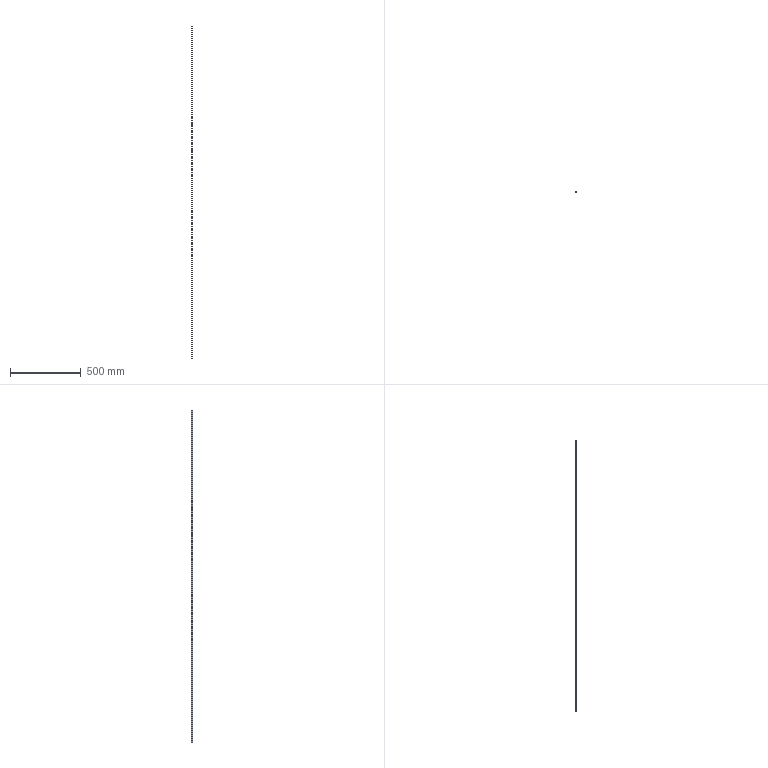Part | SolidWorks | features BaseBody 1 | 1 solid | 6 faces | box 1.5 x 10 x 2344 mm | volume 35160 mm3 | plane 6
STEP:
#1=CARTESIAN_POINT('',(0.75,5.,2344.));
#2=VERTEX_POINT('',#1);
#3=CARTESIAN_POINT('',(0.75,5.,0.));
#4=VERTEX_POINT('',#3);
#5=CARTESIAN_POINT('',(0.75,5.,2344.));
#6=DIRECTION('',(0.,0.,-1.));
#7=VECTOR('',#6,1000.);
#8=LINE('',#5,#7);
#9=EDGE_CURVE('',#2,#4,#8,.T.);
#10=ORIENTED_EDGE('',*,*,#9,.F.);
#11=CARTESIAN_POINT('',(0.75,-5.,2344.));
#12=VERTEX_POINT('',#11);
#13=CARTESIAN_POINT('',(0.75,-5.,2344.));
#14=DIRECTION('',(0.,1.,0.));
#15=VECTOR('',#14,1000.);
#16=LINE('',#13,#15);
#17=EDGE_CURVE('',#12,#2,#16,.T.);
#18=ORIENTED_EDGE('',*,*,#17,.F.);
#19=CARTESIAN_POINT('',(0.75,-5.,0.));
#20=VERTEX_POINT('',#19);
#21=CARTESIAN_POINT('',(0.75,-5.,2344.));
#22=DIRECTION('',(0.,0.,1.));
#23=VECTOR('',#22,1000.);
#24=LINE('',#21,#23);
#25=EDGE_CURVE('',#20,#12,#24,.T.);
#26=ORIENTED_EDGE('',*,*,#25,.F.);
#27=CARTESIAN_POINT('',(0.75,-5.,0.));
#28=DIRECTION('',(0.,-1.,0.));
#29=VECTOR('',#28,1000.);
#30=LINE('',#27,#29);
#31=EDGE_CURVE('',#4,#20,#30,.T.);
#32=ORIENTED_EDGE('',*,*,#31,.F.);
#33=EDGE_LOOP('',(#10,#18,#26,#32));
#34=FACE_OUTER_BOUND('',#33,.T.);
#35=CARTESIAN_POINT('',(0.75,-5.,2344.));
#36=DIRECTION('',(-1.,0.,0.));
#37=DIRECTION('',(0.,0.,1.));
#38=AXIS2_PLACEMENT_3D('',#35,#36,#37);
#39=PLANE('',#38);
#40=ADVANCED_FACE('',(#34),#39,.F.);
#41=CARTESIAN_POINT('',(-0.75,-5.,0.));
#42=VERTEX_POINT('',#41);
#43=CARTESIAN_POINT('',(-0.75,5.,0.));
#44=VERTEX_POINT('',#43);
#45=CARTESIAN_POINT('',(-0.75,0.,0.));
#46=DIRECTION('',(0.,1.,0.));
#47=VECTOR('',#46,1000.);
#48=LINE('',#45,#47);
#49=EDGE_CURVE('',#42,#44,#48,.T.);
#50=ORIENTED_EDGE('',*,*,#49,.T.);
#51=CARTESIAN_POINT('',(0.,5.,0.));
#52=DIRECTION('',(1.,0.,0.));
#53=VECTOR('',#52,1000.);
#54=LINE('',#51,#53);
#55=EDGE_CURVE('',#44,#4,#54,.T.);
#56=ORIENTED_EDGE('',*,*,#55,.T.);
#57=ORIENTED_EDGE('',*,*,#31,.T.);
#58=CARTESIAN_POINT('',(0.,-5.,0.));
#59=DIRECTION('',(-1.,0.,0.));
#60=VECTOR('',#59,1000.);
#61=LINE('',#58,#60);
#62=EDGE_CURVE('',#20,#42,#61,.T.);
#63=ORIENTED_EDGE('',*,*,#62,.T.);
#64=EDGE_LOOP('',(#50,#56,#57,#63));
#65=FACE_OUTER_BOUND('',#64,.T.);
#66=CARTESIAN_POINT('',(0.,0.,0.));
#67=DIRECTION('',(0.,0.,-1.));
#68=DIRECTION('',(-1.,0.,0.));
#69=AXIS2_PLACEMENT_3D('',#66,#67,#68);
#70=PLANE('',#69);
#71=ADVANCED_FACE('',(#65),#70,.T.);
#72=CARTESIAN_POINT('',(-0.75,5.,2344.));
#73=VERTEX_POINT('',#72);
#74=CARTESIAN_POINT('',(-0.75,5.,2344.));
#75=DIRECTION('',(0.,0.,-1.));
#76=VECTOR('',#75,1000.);
#77=LINE('',#74,#76);
#78=EDGE_CURVE('',#73,#44,#77,.T.);
#79=ORIENTED_EDGE('',*,*,#78,.F.);
#80=CARTESIAN_POINT('',(-0.75,5.,2344.));
#81=DIRECTION('',(-1.,0.,0.));
#82=VECTOR('',#81,1000.);
#83=LINE('',#80,#82);
#84=EDGE_CURVE('',#2,#73,#83,.T.);
#85=ORIENTED_EDGE('',*,*,#84,.F.);
#86=ORIENTED_EDGE('',*,*,#9,.T.);
#87=ORIENTED_EDGE('',*,*,#55,.F.);
#88=EDGE_LOOP('',(#79,#85,#86,#87));
#89=FACE_OUTER_BOUND('',#88,.T.);
#90=CARTESIAN_POINT('',(-0.75,5.,2344.));
#91=DIRECTION('',(0.,-1.,0.));
#92=DIRECTION('',(0.,0.,-1.));
#93=AXIS2_PLACEMENT_3D('',#90,#91,#92);
#94=PLANE('',#93);
#95=ADVANCED_FACE('',(#89),#94,.F.);
#96=ORIENTED_EDGE('',*,*,#84,.T.);
#97=CARTESIAN_POINT('',(-0.75,-5.,2344.));
#98=VERTEX_POINT('',#97);
#99=CARTESIAN_POINT('',(-0.75,0.,2344.));
#100=DIRECTION('',(0.,1.,0.));
#101=VECTOR('',#100,1000.);
#102=LINE('',#99,#101);
#103=EDGE_CURVE('',#98,#73,#102,.T.);
#104=ORIENTED_EDGE('',*,*,#103,.F.);
#105=CARTESIAN_POINT('',(0.,-5.,2344.));
#106=DIRECTION('',(-1.,0.,0.));
#107=VECTOR('',#106,1000.);
#108=LINE('',#105,#107);
#109=EDGE_CURVE('',#12,#98,#108,.T.);
#110=ORIENTED_EDGE('',*,*,#109,.F.);
#111=ORIENTED_EDGE('',*,*,#17,.T.);
#112=EDGE_LOOP('',(#96,#104,#110,#111));
#113=FACE_OUTER_BOUND('',#112,.T.);
#114=CARTESIAN_POINT('',(0.,0.,2344.));
#115=DIRECTION('',(0.,0.,-1.));
#116=DIRECTION('',(-1.,0.,0.));
#117=AXIS2_PLACEMENT_3D('',#114,#115,#116);
#118=PLANE('',#117);
#119=ADVANCED_FACE('',(#113),#118,.F.);
#120=ORIENTED_EDGE('',*,*,#25,.T.);
#121=ORIENTED_EDGE('',*,*,#109,.T.);
#122=CARTESIAN_POINT('',(-0.75,-5.,2344.));
#123=DIRECTION('',(0.,0.,1.));
#124=VECTOR('',#123,1000.);
#125=LINE('',#122,#124);
#126=EDGE_CURVE('',#42,#98,#125,.T.);
#127=ORIENTED_EDGE('',*,*,#126,.F.);
#128=ORIENTED_EDGE('',*,*,#62,.F.);
#129=EDGE_LOOP('',(#120,#121,#127,#128));
#130=FACE_OUTER_BOUND('',#129,.T.);
#131=CARTESIAN_POINT('',(-0.75,-5.,2344.));
#132=DIRECTION('',(0.,1.,0.));
#133=DIRECTION('',(0.,0.,1.));
#134=AXIS2_PLACEMENT_3D('',#131,#132,#133);
#135=PLANE('',#134);
#136=ADVANCED_FACE('',(#130),#135,.F.);
#137=ORIENTED_EDGE('',*,*,#126,.T.);
#138=ORIENTED_EDGE('',*,*,#103,.T.);
#139=ORIENTED_EDGE('',*,*,#78,.T.);
#140=ORIENTED_EDGE('',*,*,#49,.F.);
#141=EDGE_LOOP('',(#137,#138,#139,#140));
#142=FACE_OUTER_BOUND('',#141,.T.);
#143=CARTESIAN_POINT('',(-0.75,-5.,2344.));
#144=DIRECTION('',(1.,0.,0.));
#145=DIRECTION('',(0.,0.,-1.));
#146=AXIS2_PLACEMENT_3D('',#143,#144,#145);
#147=PLANE('',#146);
#148=ADVANCED_FACE('',(#142),#147,.F.);
#149=CLOSED_SHELL('',(#40,#71,#95,#119,#136,#148));
#150=MANIFOLD_SOLID_BREP('',#149);
#151=CARTESIAN_POINT('',(0.,0.,0.));
#152=DIRECTION('',(0.,0.,1.));
#153=DIRECTION('',(1.,0.,0.));
#154=AXIS2_PLACEMENT_3D('',#151,#152,#153);
#155=(LENGTH_UNIT()NAMED_UNIT(*)SI_UNIT(.MILLI.,.METRE.));
#156=UNCERTAINTY_MEASURE_WITH_UNIT(LENGTH_MEASURE(0.00001),#155,'','');
#157=(NAMED_UNIT(*)PLANE_ANGLE_UNIT()SI_UNIT($,.RADIAN.));
#158=(NAMED_UNIT(*)SI_UNIT($,.STERADIAN.)SOLID_ANGLE_UNIT());
#159=(GEOMETRIC_REPRESENTATION_CONTEXT(3)GLOBAL_UNCERTAINTY_ASSIGNED_CONTEXT((#156))GLOBAL_UNIT_ASSIGNED_CONTEXT((#155,#157,#158))REPRESENTATION_CONTEXT('',''));
#160=ADVANCED_BREP_SHAPE_REPRESENTATION('',(#150,#154),#159);